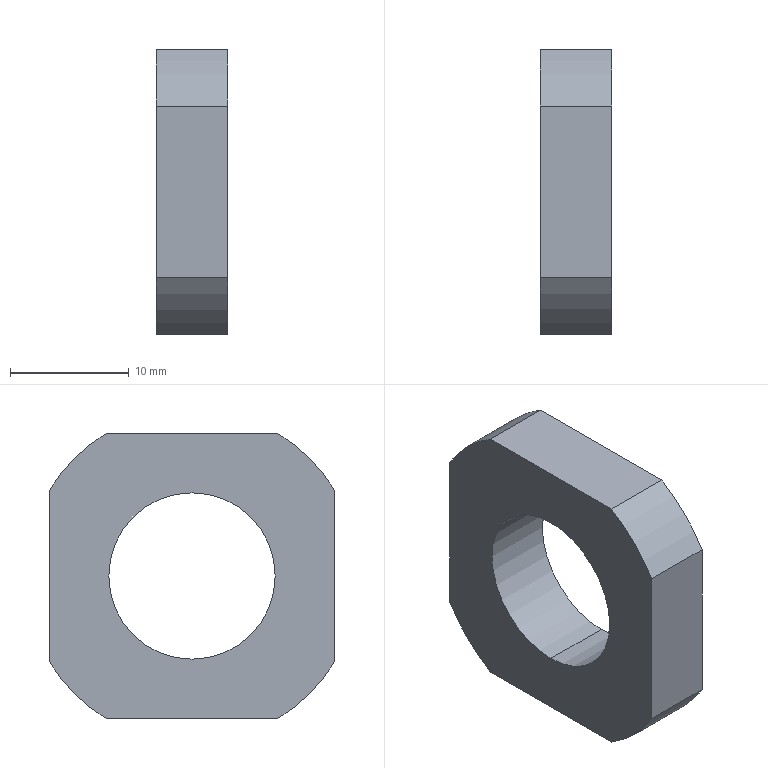Part | STEP file | PN_0053 locking nut | 1 solid | 12 faces | box 6 x 24 x 24 mm | volume 2302 mm3 | cylinder 6 | plane 6 | commonest cylinder face diameters 28 x4 14 x2
STEP:
#1=CARTESIAN_POINT('',(0.,0.,0.));
#2=DIRECTION('',(0.,0.,1.));
#3=DIRECTION('',(1.,0.,0.));
#4=AXIS2_PLACEMENT_3D('',#1,#2,#3);
#5=CARTESIAN_POINT('',(0.,0.,7.));
#6=VERTEX_POINT('',#5);
#7=CARTESIAN_POINT('',(-6.,0.,7.));
#8=VERTEX_POINT('',#7);
#9=CARTESIAN_POINT('',(0.,0.,7.));
#10=DIRECTION('',(-1.,0.,0.));
#11=VECTOR('',#10,1.);
#12=LINE('',#9,#11);
#13=CARTESIAN_POINT('',(0.,0.,0.));
#14=DIRECTION('',(-1.,0.,0.));
#15=DIRECTION('',(0.,0.,1.));
#16=AXIS2_PLACEMENT_3D('',#13,#14,#15);
#17=CYLINDRICAL_SURFACE('',#16,7.);
#18=CARTESIAN_POINT('',(6.283,0.));
#19=DIRECTION('',(0.,1.));
#20=VECTOR('',#19,1.);
#21=LINE('',#18,#20);
#22=(GEOMETRIC_REPRESENTATION_CONTEXT(2)PARAMETRIC_REPRESENTATION_CONTEXT()REPRESENTATION_CONTEXT('',''));
#23=DEFINITIONAL_REPRESENTATION('',(#21),#22);
#24=PCURVE('',#17,#23);
#25=CARTESIAN_POINT('',(0.,0.,0.));
#26=DIRECTION('',(-1.,0.,0.));
#27=DIRECTION('',(0.,0.,1.));
#28=AXIS2_PLACEMENT_3D('',#25,#26,#27);
#29=CYLINDRICAL_SURFACE('',#28,7.);
#30=CARTESIAN_POINT('',(0.,0.));
#31=DIRECTION('',(0.,1.));
#32=VECTOR('',#31,1.);
#33=LINE('',#30,#32);
#34=(GEOMETRIC_REPRESENTATION_CONTEXT(2)PARAMETRIC_REPRESENTATION_CONTEXT()REPRESENTATION_CONTEXT('',''));
#35=DEFINITIONAL_REPRESENTATION('',(#33),#34);
#36=PCURVE('',#29,#35);
#37=SURFACE_CURVE('',#12,(#24,#36),.PCURVE_S1.);
#38=EDGE_CURVE('',#6,#8,#37,.T.);
#39=ORIENTED_EDGE('',*,*,#38,.T.);
#40=CARTESIAN_POINT('',(-6.,0.,-7.));
#41=VERTEX_POINT('',#40);
#42=CARTESIAN_POINT('',(-6.,0.,0.));
#43=DIRECTION('',(1.,0.,0.));
#44=DIRECTION('',(0.,0.,-1.));
#45=AXIS2_PLACEMENT_3D('',#42,#43,#44);
#46=CIRCLE('',#45,7.);
#47=CARTESIAN_POINT('',(9.425,6.));
#48=DIRECTION('',(-1.,0.));
#49=VECTOR('',#48,1.);
#50=LINE('',#47,#49);
#51=(GEOMETRIC_REPRESENTATION_CONTEXT(2)PARAMETRIC_REPRESENTATION_CONTEXT()REPRESENTATION_CONTEXT('',''));
#52=DEFINITIONAL_REPRESENTATION('',(#50),#51);
#53=PCURVE('',#17,#52);
#54=CARTESIAN_POINT('',(-6.,14.,0.));
#55=DIRECTION('',(-1.,0.,0.));
#56=DIRECTION('',(0.,0.,1.));
#57=AXIS2_PLACEMENT_3D('',#54,#55,#56);
#58=PLANE('',#57);
#59=CARTESIAN_POINT('',(-7.,-14.));
#60=CARTESIAN_POINT('',(-7.,-1.876));
#61=CARTESIAN_POINT('',(3.5,-7.938));
#62=CARTESIAN_POINT('',(14.,-14.));
#63=CARTESIAN_POINT('',(3.5,-20.062));
#64=CARTESIAN_POINT('',(-7.,-26.124));
#65=CARTESIAN_POINT('',(-7.,-14.));
#66=(BOUNDED_CURVE()B_SPLINE_CURVE(2,(#59,#60,#61,#62,#63,#64,#65),.UNSPECIFIED.,.T.,.F.)B_SPLINE_CURVE_WITH_KNOTS((1,2,2,2,2,1),(-2.094,0.,2.094,4.189,6.283,8.378),.UNSPECIFIED.)CURVE()GEOMETRIC_REPRESENTATION_ITEM()RATIONAL_B_SPLINE_CURVE((1.,0.5,1.,0.5,1.,0.5,1.))REPRESENTATION_ITEM(''));
#67=(GEOMETRIC_REPRESENTATION_CONTEXT(2)PARAMETRIC_REPRESENTATION_CONTEXT()REPRESENTATION_CONTEXT('',''));
#68=DEFINITIONAL_REPRESENTATION('',(#66),#67);
#69=PCURVE('',#58,#68);
#70=SURFACE_CURVE('',#46,(#53,#69),.PCURVE_S1.);
#71=EDGE_CURVE('',#8,#41,#70,.T.);
#72=ORIENTED_EDGE('',*,*,#71,.T.);
#73=CARTESIAN_POINT('',(0.,0.,-7.));
#74=VERTEX_POINT('',#73);
#75=CARTESIAN_POINT('',(0.,0.,-7.));
#76=DIRECTION('',(-1.,0.,0.));
#77=VECTOR('',#76,1.);
#78=LINE('',#75,#77);
#79=CARTESIAN_POINT('',(3.142,0.));
#80=DIRECTION('',(0.,1.));
#81=VECTOR('',#80,1.);
#82=LINE('',#79,#81);
#83=(GEOMETRIC_REPRESENTATION_CONTEXT(2)PARAMETRIC_REPRESENTATION_CONTEXT()REPRESENTATION_CONTEXT('',''));
#84=DEFINITIONAL_REPRESENTATION('',(#82),#83);
#85=PCURVE('',#17,#84);
#86=CARTESIAN_POINT('',(3.142,0.));
#87=DIRECTION('',(0.,1.));
#88=VECTOR('',#87,1.);
#89=LINE('',#86,#88);
#90=(GEOMETRIC_REPRESENTATION_CONTEXT(2)PARAMETRIC_REPRESENTATION_CONTEXT()REPRESENTATION_CONTEXT('',''));
#91=DEFINITIONAL_REPRESENTATION('',(#89),#90);
#92=PCURVE('',#29,#91);
#93=SURFACE_CURVE('',#78,(#85,#92),.PCURVE_S1.);
#94=EDGE_CURVE('',#74,#41,#93,.T.);
#95=ORIENTED_EDGE('',*,*,#94,.F.);
#96=CARTESIAN_POINT('',(0.,0.,0.));
#97=DIRECTION('',(1.,0.,0.));
#98=DIRECTION('',(0.,0.,-1.));
#99=AXIS2_PLACEMENT_3D('',#96,#97,#98);
#100=CIRCLE('',#99,7.);
#101=CARTESIAN_POINT('',(9.425,0.));
#102=DIRECTION('',(-1.,0.));
#103=VECTOR('',#102,1.);
#104=LINE('',#101,#103);
#105=(GEOMETRIC_REPRESENTATION_CONTEXT(2)PARAMETRIC_REPRESENTATION_CONTEXT()REPRESENTATION_CONTEXT('',''));
#106=DEFINITIONAL_REPRESENTATION('',(#104),#105);
#107=PCURVE('',#17,#106);
#108=CARTESIAN_POINT('',(0.,0.,0.));
#109=DIRECTION('',(1.,0.,0.));
#110=DIRECTION('',(0.,0.,-1.));
#111=AXIS2_PLACEMENT_3D('',#108,#109,#110);
#112=PLANE('',#111);
#113=CARTESIAN_POINT('',(0.,0.));
#114=DIRECTION('',(1.,0.));
#115=AXIS2_PLACEMENT_2D('',#113,#114);
#116=CIRCLE('',#115,7.);
#117=(GEOMETRIC_REPRESENTATION_CONTEXT(2)PARAMETRIC_REPRESENTATION_CONTEXT()REPRESENTATION_CONTEXT('',''));
#118=DEFINITIONAL_REPRESENTATION('',(#116),#117);
#119=PCURVE('',#112,#118);
#120=SURFACE_CURVE('',#100,(#107,#119),.PCURVE_S1.);
#121=EDGE_CURVE('',#6,#74,#120,.T.);
#122=ORIENTED_EDGE('',*,*,#121,.F.);
#123=EDGE_LOOP('',(#39,#72,#95,#122));
#124=FACE_BOUND('',#123,.F.);
#125=ADVANCED_FACE('',(#124),#17,.F.);
#126=CARTESIAN_POINT('',(0.,7.211,12.));
#127=VERTEX_POINT('',#126);
#128=CARTESIAN_POINT('',(-6.,7.211,12.));
#129=VERTEX_POINT('',#128);
#130=CARTESIAN_POINT('',(0.,7.211,12.));
#131=DIRECTION('',(-1.,0.,0.));
#132=VECTOR('',#131,1.);
#133=LINE('',#130,#132);
#134=CARTESIAN_POINT('',(0.,0.,0.));
#135=DIRECTION('',(1.,0.,0.));
#136=DIRECTION('',(0.,0.,-1.));
#137=AXIS2_PLACEMENT_3D('',#134,#135,#136);
#138=CYLINDRICAL_SURFACE('',#137,14.);
#139=CARTESIAN_POINT('',(2.6,0.));
#140=DIRECTION('',(0.,-1.));
#141=VECTOR('',#140,1.);
#142=LINE('',#139,#141);
#143=(GEOMETRIC_REPRESENTATION_CONTEXT(2)PARAMETRIC_REPRESENTATION_CONTEXT()REPRESENTATION_CONTEXT('',''));
#144=DEFINITIONAL_REPRESENTATION('',(#142),#143);
#145=PCURVE('',#138,#144);
#146=CARTESIAN_POINT('',(0.,17.205,12.));
#147=DIRECTION('',(0.,0.,-1.));
#148=DIRECTION('',(0.,1.,0.));
#149=AXIS2_PLACEMENT_3D('',#146,#147,#148);
#150=PLANE('',#149);
#151=CARTESIAN_POINT('',(-9.994,0.));
#152=DIRECTION('',(0.,-1.));
#153=VECTOR('',#152,1.);
#154=LINE('',#151,#153);
#155=(GEOMETRIC_REPRESENTATION_CONTEXT(2)PARAMETRIC_REPRESENTATION_CONTEXT()REPRESENTATION_CONTEXT('',''));
#156=DEFINITIONAL_REPRESENTATION('',(#154),#155);
#157=PCURVE('',#150,#156);
#158=SURFACE_CURVE('',#133,(#145,#157),.PCURVE_S1.);
#159=EDGE_CURVE('',#127,#129,#158,.T.);
#160=ORIENTED_EDGE('',*,*,#159,.F.);
#161=CARTESIAN_POINT('',(0.,12.,7.211));
#162=VERTEX_POINT('',#161);
#163=CARTESIAN_POINT('',(0.,0.,0.));
#164=DIRECTION('',(1.,0.,0.));
#165=DIRECTION('',(0.,0.,-1.));
#166=AXIS2_PLACEMENT_3D('',#163,#164,#165);
#167=CIRCLE('',#166,14.);
#168=CARTESIAN_POINT('',(0.,0.));
#169=DIRECTION('',(1.,0.));
#170=VECTOR('',#169,1.);
#171=LINE('',#168,#170);
#172=(GEOMETRIC_REPRESENTATION_CONTEXT(2)PARAMETRIC_REPRESENTATION_CONTEXT()REPRESENTATION_CONTEXT('',''));
#173=DEFINITIONAL_REPRESENTATION('',(#171),#172);
#174=PCURVE('',#138,#173);
#175=CARTESIAN_POINT('',(0.,0.));
#176=DIRECTION('',(1.,0.));
#177=AXIS2_PLACEMENT_2D('',#175,#176);
#178=CIRCLE('',#177,14.);
#179=(GEOMETRIC_REPRESENTATION_CONTEXT(2)PARAMETRIC_REPRESENTATION_CONTEXT()REPRESENTATION_CONTEXT('',''));
#180=DEFINITIONAL_REPRESENTATION('',(#178),#179);
#181=PCURVE('',#112,#180);
#182=SURFACE_CURVE('',#167,(#174,#181),.PCURVE_S1.);
#183=EDGE_CURVE('',#162,#127,#182,.T.);
#184=ORIENTED_EDGE('',*,*,#183,.F.);
#185=CARTESIAN_POINT('',(-6.,12.,7.211));
#186=VERTEX_POINT('',#185);
#187=CARTESIAN_POINT('',(0.,12.,7.211));
#188=DIRECTION('',(1.,0.,0.));
#189=VECTOR('',#188,1.);
#190=LINE('',#187,#189);
#191=CARTESIAN_POINT('',(2.112,0.));
#192=DIRECTION('',(0.,1.));
#193=VECTOR('',#192,1.);
#194=LINE('',#191,#193);
#195=(GEOMETRIC_REPRESENTATION_CONTEXT(2)PARAMETRIC_REPRESENTATION_CONTEXT()REPRESENTATION_CONTEXT('',''));
#196=DEFINITIONAL_REPRESENTATION('',(#194),#195);
#197=PCURVE('',#138,#196);
#198=CARTESIAN_POINT('',(0.,12.,-20.296));
#199=DIRECTION('',(0.,-1.,0.));
#200=DIRECTION('',(0.,0.,-1.));
#201=AXIS2_PLACEMENT_3D('',#198,#199,#200);
#202=PLANE('',#201);
#203=CARTESIAN_POINT('',(-27.507,0.));
#204=DIRECTION('',(0.,1.));
#205=VECTOR('',#204,1.);
#206=LINE('',#203,#205);
#207=(GEOMETRIC_REPRESENTATION_CONTEXT(2)PARAMETRIC_REPRESENTATION_CONTEXT()REPRESENTATION_CONTEXT('',''));
#208=DEFINITIONAL_REPRESENTATION('',(#206),#207);
#209=PCURVE('',#202,#208);
#210=SURFACE_CURVE('',#190,(#197,#209),.PCURVE_S1.);
#211=EDGE_CURVE('',#186,#162,#210,.T.);
#212=ORIENTED_EDGE('',*,*,#211,.F.);
#213=CARTESIAN_POINT('',(-6.,0.,0.));
#214=DIRECTION('',(1.,0.,0.));
#215=DIRECTION('',(0.,0.,-1.));
#216=AXIS2_PLACEMENT_3D('',#213,#214,#215);
#217=CIRCLE('',#216,14.);
#218=CARTESIAN_POINT('',(0.,-6.));
#219=DIRECTION('',(1.,0.));
#220=VECTOR('',#219,1.);
#221=LINE('',#218,#220);
#222=(GEOMETRIC_REPRESENTATION_CONTEXT(2)PARAMETRIC_REPRESENTATION_CONTEXT()REPRESENTATION_CONTEXT('',''));
#223=DEFINITIONAL_REPRESENTATION('',(#221),#222);
#224=PCURVE('',#138,#223);
#225=CARTESIAN_POINT('',(-14.,-14.));
#226=CARTESIAN_POINT('',(-14.,10.249));
#227=CARTESIAN_POINT('',(7.,-1.876));
#228=CARTESIAN_POINT('',(28.,-14.));
#229=CARTESIAN_POINT('',(7.,-26.124));
#230=CARTESIAN_POINT('',(-14.,-38.249));
#231=CARTESIAN_POINT('',(-14.,-14.));
#232=(BOUNDED_CURVE()B_SPLINE_CURVE(2,(#225,#226,#227,#228,#229,#230,#231),.UNSPECIFIED.,.T.,.F.)B_SPLINE_CURVE_WITH_KNOTS((1,2,2,2,2,1),(-2.094,0.,2.094,4.189,6.283,8.378),.UNSPECIFIED.)CURVE()GEOMETRIC_REPRESENTATION_ITEM()RATIONAL_B_SPLINE_CURVE((1.,0.5,1.,0.5,1.,0.5,1.))REPRESENTATION_ITEM(''));
#233=(GEOMETRIC_REPRESENTATION_CONTEXT(2)PARAMETRIC_REPRESENTATION_CONTEXT()REPRESENTATION_CONTEXT('',''));
#234=DEFINITIONAL_REPRESENTATION('',(#232),#233);
#235=PCURVE('',#58,#234);
#236=SURFACE_CURVE('',#217,(#224,#235),.PCURVE_S1.);
#237=EDGE_CURVE('',#186,#129,#236,.T.);
#238=ORIENTED_EDGE('',*,*,#237,.T.);
#239=EDGE_LOOP('',(#160,#184,#212,#238));
#240=FACE_BOUND('',#239,.T.);
#241=ADVANCED_FACE('',(#240),#138,.T.);
#242=CARTESIAN_POINT('',(0.,-7.211,-12.));
#243=VERTEX_POINT('',#242);
#244=CARTESIAN_POINT('',(-6.,-7.211,-12.));
#245=VERTEX_POINT('',#244);
#246=CARTESIAN_POINT('',(0.,-7.211,-12.));
#247=DIRECTION('',(-1.,0.,0.));
#248=VECTOR('',#247,1.);
#249=LINE('',#246,#248);
#250=CARTESIAN_POINT('',(0.,0.,0.));
#251=DIRECTION('',(1.,0.,0.));
#252=DIRECTION('',(0.,0.,-1.));
#253=AXIS2_PLACEMENT_3D('',#250,#251,#252);
#254=CYLINDRICAL_SURFACE('',#253,14.);
#255=CARTESIAN_POINT('',(5.742,0.));
#256=DIRECTION('',(0.,-1.));
#257=VECTOR('',#256,1.);
#258=LINE('',#255,#257);
#259=(GEOMETRIC_REPRESENTATION_CONTEXT(2)PARAMETRIC_REPRESENTATION_CONTEXT()REPRESENTATION_CONTEXT('',''));
#260=DEFINITIONAL_REPRESENTATION('',(#258),#259);
#261=PCURVE('',#254,#260);
#262=CARTESIAN_POINT('',(0.,17.205,-12.));
#263=DIRECTION('',(0.,0.,1.));
#264=DIRECTION('',(0.,-1.,0.));
#265=AXIS2_PLACEMENT_3D('',#262,#263,#264);
#266=PLANE('',#265);
#267=CARTESIAN_POINT('',(24.416,0.));
#268=DIRECTION('',(0.,-1.));
#269=VECTOR('',#268,1.);
#270=LINE('',#267,#269);
#271=(GEOMETRIC_REPRESENTATION_CONTEXT(2)PARAMETRIC_REPRESENTATION_CONTEXT()REPRESENTATION_CONTEXT('',''));
#272=DEFINITIONAL_REPRESENTATION('',(#270),#271);
#273=PCURVE('',#266,#272);
#274=SURFACE_CURVE('',#249,(#261,#273),.PCURVE_S1.);
#275=EDGE_CURVE('',#243,#245,#274,.T.);
#276=ORIENTED_EDGE('',*,*,#275,.F.);
#277=CARTESIAN_POINT('',(0.,-12.,-7.211));
#278=VERTEX_POINT('',#277);
#279=CARTESIAN_POINT('',(0.,0.,0.));
#280=DIRECTION('',(1.,0.,0.));
#281=DIRECTION('',(0.,0.,-1.));
#282=AXIS2_PLACEMENT_3D('',#279,#280,#281);
#283=CIRCLE('',#282,14.);
#284=CARTESIAN_POINT('',(0.,0.));
#285=DIRECTION('',(1.,0.));
#286=VECTOR('',#285,1.);
#287=LINE('',#284,#286);
#288=(GEOMETRIC_REPRESENTATION_CONTEXT(2)PARAMETRIC_REPRESENTATION_CONTEXT()REPRESENTATION_CONTEXT('',''));
#289=DEFINITIONAL_REPRESENTATION('',(#287),#288);
#290=PCURVE('',#254,#289);
#291=CARTESIAN_POINT('',(0.,0.));
#292=DIRECTION('',(1.,0.));
#293=AXIS2_PLACEMENT_2D('',#291,#292);
#294=CIRCLE('',#293,14.);
#295=(GEOMETRIC_REPRESENTATION_CONTEXT(2)PARAMETRIC_REPRESENTATION_CONTEXT()REPRESENTATION_CONTEXT('',''));
#296=DEFINITIONAL_REPRESENTATION('',(#294),#295);
#297=PCURVE('',#112,#296);
#298=SURFACE_CURVE('',#283,(#290,#297),.PCURVE_S1.);
#299=EDGE_CURVE('',#278,#243,#298,.T.);
#300=ORIENTED_EDGE('',*,*,#299,.F.);
#301=CARTESIAN_POINT('',(-6.,-12.,-7.211));
#302=VERTEX_POINT('',#301);
#303=CARTESIAN_POINT('',(0.,-12.,-7.211));
#304=DIRECTION('',(1.,0.,0.));
#305=VECTOR('',#304,1.);
#306=LINE('',#303,#305);
#307=CARTESIAN_POINT('',(5.253,0.));
#308=DIRECTION('',(0.,1.));
#309=VECTOR('',#308,1.);
#310=LINE('',#307,#309);
#311=(GEOMETRIC_REPRESENTATION_CONTEXT(2)PARAMETRIC_REPRESENTATION_CONTEXT()REPRESENTATION_CONTEXT('',''));
#312=DEFINITIONAL_REPRESENTATION('',(#310),#311);
#313=PCURVE('',#254,#312);
#314=CARTESIAN_POINT('',(0.,-12.,-20.296));
#315=DIRECTION('',(0.,1.,0.));
#316=DIRECTION('',(0.,0.,1.));
#317=AXIS2_PLACEMENT_3D('',#314,#315,#316);
#318=PLANE('',#317);
#319=CARTESIAN_POINT('',(13.085,0.));
#320=DIRECTION('',(0.,1.));
#321=VECTOR('',#320,1.);
#322=LINE('',#319,#321);
#323=(GEOMETRIC_REPRESENTATION_CONTEXT(2)PARAMETRIC_REPRESENTATION_CONTEXT()REPRESENTATION_CONTEXT('',''));
#324=DEFINITIONAL_REPRESENTATION('',(#322),#323);
#325=PCURVE('',#318,#324);
#326=SURFACE_CURVE('',#306,(#313,#325),.PCURVE_S1.);
#327=EDGE_CURVE('',#302,#278,#326,.T.);
#328=ORIENTED_EDGE('',*,*,#327,.F.);
#329=CARTESIAN_POINT('',(-6.,0.,0.));
#330=DIRECTION('',(1.,0.,0.));
#331=DIRECTION('',(0.,0.,-1.));
#332=AXIS2_PLACEMENT_3D('',#329,#330,#331);
#333=CIRCLE('',#332,14.);
#334=CARTESIAN_POINT('',(0.,-6.));
#335=DIRECTION('',(1.,0.));
#336=VECTOR('',#335,1.);
#337=LINE('',#334,#336);
#338=(GEOMETRIC_REPRESENTATION_CONTEXT(2)PARAMETRIC_REPRESENTATION_CONTEXT()REPRESENTATION_CONTEXT('',''));
#339=DEFINITIONAL_REPRESENTATION('',(#337),#338);
#340=PCURVE('',#254,#339);
#341=CARTESIAN_POINT('',(-14.,-14.));
#342=CARTESIAN_POINT('',(-14.,10.249));
#343=CARTESIAN_POINT('',(7.,-1.876));
#344=CARTESIAN_POINT('',(28.,-14.));
#345=CARTESIAN_POINT('',(7.,-26.124));
#346=CARTESIAN_POINT('',(-14.,-38.249));
#347=CARTESIAN_POINT('',(-14.,-14.));
#348=(BOUNDED_CURVE()B_SPLINE_CURVE(2,(#341,#342,#343,#344,#345,#346,#347),.UNSPECIFIED.,.T.,.F.)B_SPLINE_CURVE_WITH_KNOTS((1,2,2,2,2,1),(-2.094,0.,2.094,4.189,6.283,8.378),.UNSPECIFIED.)CURVE()GEOMETRIC_REPRESENTATION_ITEM()RATIONAL_B_SPLINE_CURVE((1.,0.5,1.,0.5,1.,0.5,1.))REPRESENTATION_ITEM(''));
#349=(GEOMETRIC_REPRESENTATION_CONTEXT(2)PARAMETRIC_REPRESENTATION_CONTEXT()REPRESENTATION_CONTEXT('',''));
#350=DEFINITIONAL_REPRESENTATION('',(#348),#349);
#351=PCURVE('',#58,#350);
#352=SURFACE_CURVE('',#333,(#340,#351),.PCURVE_S1.);
#353=EDGE_CURVE('',#302,#245,#352,.T.);
#354=ORIENTED_EDGE('',*,*,#353,.T.);
#355=EDGE_LOOP('',(#276,#300,#328,#354));
#356=FACE_BOUND('',#355,.T.);
#357=ADVANCED_FACE('',(#356),#254,.T.);
#358=CARTESIAN_POINT('',(-6.,-7.211,12.));
#359=VERTEX_POINT('',#358);
#360=CARTESIAN_POINT('',(0.,-7.211,12.));
#361=VERTEX_POINT('',#360);
#362=CARTESIAN_POINT('',(0.,-7.211,12.));
#363=DIRECTION('',(1.,0.,0.));
#364=VECTOR('',#363,1.);
#365=LINE('',#362,#364);
#366=CARTESIAN_POINT('',(0.,0.,0.));
#367=DIRECTION('',(1.,0.,0.));
#368=DIRECTION('',(0.,0.,-1.));
#369=AXIS2_PLACEMENT_3D('',#366,#367,#368);
#370=CYLINDRICAL_SURFACE('',#369,14.);
#371=CARTESIAN_POINT('',(3.683,0.));
#372=DIRECTION('',(0.,1.));
#373=VECTOR('',#372,1.);
#374=LINE('',#371,#373);
#375=(GEOMETRIC_REPRESENTATION_CONTEXT(2)PARAMETRIC_REPRESENTATION_CONTEXT()REPRESENTATION_CONTEXT('',''));
#376=DEFINITIONAL_REPRESENTATION('',(#374),#375);
#377=PCURVE('',#370,#376);
#378=CARTESIAN_POINT('',(-24.416,0.));
#379=DIRECTION('',(0.,1.));
#380=VECTOR('',#379,1.);
#381=LINE('',#378,#380);
#382=(GEOMETRIC_REPRESENTATION_CONTEXT(2)PARAMETRIC_REPRESENTATION_CONTEXT()REPRESENTATION_CONTEXT('',''));
#383=DEFINITIONAL_REPRESENTATION('',(#381),#382);
#384=PCURVE('',#150,#383);
#385=SURFACE_CURVE('',#365,(#377,#384),.PCURVE_S1.);
#386=EDGE_CURVE('',#359,#361,#385,.T.);
#387=ORIENTED_EDGE('',*,*,#386,.F.);
#388=CARTESIAN_POINT('',(-6.,-12.,7.211));
#389=VERTEX_POINT('',#388);
#390=CARTESIAN_POINT('',(-6.,0.,0.));
#391=DIRECTION('',(1.,0.,0.));
#392=DIRECTION('',(0.,0.,-1.));
#393=AXIS2_PLACEMENT_3D('',#390,#391,#392);
#394=CIRCLE('',#393,14.);
#395=CARTESIAN_POINT('',(0.,-6.));
#396=DIRECTION('',(1.,0.));
#397=VECTOR('',#396,1.);
#398=LINE('',#395,#397);
#399=(GEOMETRIC_REPRESENTATION_CONTEXT(2)PARAMETRIC_REPRESENTATION_CONTEXT()REPRESENTATION_CONTEXT('',''));
#400=DEFINITIONAL_REPRESENTATION('',(#398),#399);
#401=PCURVE('',#370,#400);
#402=CARTESIAN_POINT('',(-14.,-14.));
#403=CARTESIAN_POINT('',(-14.,10.249));
#404=CARTESIAN_POINT('',(7.,-1.876));
#405=CARTESIAN_POINT('',(28.,-14.));
#406=CARTESIAN_POINT('',(7.,-26.124));
#407=CARTESIAN_POINT('',(-14.,-38.249));
#408=CARTESIAN_POINT('',(-14.,-14.));
#409=(BOUNDED_CURVE()B_SPLINE_CURVE(2,(#402,#403,#404,#405,#406,#407,#408),.UNSPECIFIED.,.T.,.F.)B_SPLINE_CURVE_WITH_KNOTS((1,2,2,2,2,1),(-2.094,0.,2.094,4.189,6.283,8.378),.UNSPECIFIED.)CURVE()GEOMETRIC_REPRESENTATION_ITEM()RATIONAL_B_SPLINE_CURVE((1.,0.5,1.,0.5,1.,0.5,1.))REPRESENTATION_ITEM(''));
#410=(GEOMETRIC_REPRESENTATION_CONTEXT(2)PARAMETRIC_REPRESENTATION_CONTEXT()REPRESENTATION_CONTEXT('',''));
#411=DEFINITIONAL_REPRESENTATION('',(#409),#410);
#412=PCURVE('',#58,#411);
#413=SURFACE_CURVE('',#394,(#401,#412),.PCURVE_S1.);
#414=EDGE_CURVE('',#359,#389,#413,.T.);
#415=ORIENTED_EDGE('',*,*,#414,.T.);
#416=CARTESIAN_POINT('',(0.,-12.,7.211));
#417=VERTEX_POINT('',#416);
#418=CARTESIAN_POINT('',(0.,-12.,7.211));
#419=DIRECTION('',(-1.,0.,0.));
#420=VECTOR('',#419,1.);
#421=LINE('',#418,#420);
#422=CARTESIAN_POINT('',(4.171,0.));
#423=DIRECTION('',(0.,-1.));
#424=VECTOR('',#423,1.);
#425=LINE('',#422,#424);
#426=(GEOMETRIC_REPRESENTATION_CONTEXT(2)PARAMETRIC_REPRESENTATION_CONTEXT()REPRESENTATION_CONTEXT('',''));
#427=DEFINITIONAL_REPRESENTATION('',(#425),#426);
#428=PCURVE('',#370,#427);
#429=CARTESIAN_POINT('',(27.507,0.));
#430=DIRECTION('',(0.,-1.));
#431=VECTOR('',#430,1.);
#432=LINE('',#429,#431);
#433=(GEOMETRIC_REPRESENTATION_CONTEXT(2)PARAMETRIC_REPRESENTATION_CONTEXT()REPRESENTATION_CONTEXT('',''));
#434=DEFINITIONAL_REPRESENTATION('',(#432),#433);
#435=PCURVE('',#318,#434);
#436=SURFACE_CURVE('',#421,(#428,#435),.PCURVE_S1.);
#437=EDGE_CURVE('',#417,#389,#436,.T.);
#438=ORIENTED_EDGE('',*,*,#437,.F.);
#439=CARTESIAN_POINT('',(0.,0.,0.));
#440=DIRECTION('',(1.,0.,0.));
#441=DIRECTION('',(0.,0.,-1.));
#442=AXIS2_PLACEMENT_3D('',#439,#440,#441);
#443=CIRCLE('',#442,14.);
#444=CARTESIAN_POINT('',(0.,0.));
#445=DIRECTION('',(1.,0.));
#446=VECTOR('',#445,1.);
#447=LINE('',#444,#446);
#448=(GEOMETRIC_REPRESENTATION_CONTEXT(2)PARAMETRIC_REPRESENTATION_CONTEXT()REPRESENTATION_CONTEXT('',''));
#449=DEFINITIONAL_REPRESENTATION('',(#447),#448);
#450=PCURVE('',#370,#449);
#451=CARTESIAN_POINT('',(0.,0.));
#452=DIRECTION('',(1.,0.));
#453=AXIS2_PLACEMENT_2D('',#451,#452);
#454=CIRCLE('',#453,14.);
#455=(GEOMETRIC_REPRESENTATION_CONTEXT(2)PARAMETRIC_REPRESENTATION_CONTEXT()REPRESENTATION_CONTEXT('',''));
#456=DEFINITIONAL_REPRESENTATION('',(#454),#455);
#457=PCURVE('',#112,#456);
#458=SURFACE_CURVE('',#443,(#450,#457),.PCURVE_S1.);
#459=EDGE_CURVE('',#361,#417,#458,.T.);
#460=ORIENTED_EDGE('',*,*,#459,.F.);
#461=EDGE_LOOP('',(#387,#415,#438,#460));
#462=FACE_BOUND('',#461,.T.);
#463=ADVANCED_FACE('',(#462),#370,.T.);
#464=CARTESIAN_POINT('',(0.,17.205,12.));
#465=DIRECTION('',(0.,-1.,0.));
#466=VECTOR('',#465,1.);
#467=LINE('',#464,#466);
#468=CARTESIAN_POINT('',(-12.,17.205));
#469=DIRECTION('',(0.,-1.));
#470=VECTOR('',#469,1.);
#471=LINE('',#468,#470);
#472=(GEOMETRIC_REPRESENTATION_CONTEXT(2)PARAMETRIC_REPRESENTATION_CONTEXT()REPRESENTATION_CONTEXT('',''));
#473=DEFINITIONAL_REPRESENTATION('',(#471),#472);
#474=PCURVE('',#112,#473);
#475=CARTESIAN_POINT('',(0.,0.));
#476=DIRECTION('',(-1.,0.));
#477=VECTOR('',#476,1.);
#478=LINE('',#475,#477);
#479=(GEOMETRIC_REPRESENTATION_CONTEXT(2)PARAMETRIC_REPRESENTATION_CONTEXT()REPRESENTATION_CONTEXT('',''));
#480=DEFINITIONAL_REPRESENTATION('',(#478),#479);
#481=PCURVE('',#150,#480);
#482=SURFACE_CURVE('',#467,(#474,#481),.PCURVE_S1.);
#483=EDGE_CURVE('',#127,#361,#482,.T.);
#484=ORIENTED_EDGE('',*,*,#483,.T.);
#485=ORIENTED_EDGE('',*,*,#459,.T.);
#486=CARTESIAN_POINT('',(0.,-12.,-20.296));
#487=DIRECTION('',(0.,0.,-1.));
#488=VECTOR('',#487,1.);
#489=LINE('',#486,#488);
#490=CARTESIAN_POINT('',(20.296,-12.));
#491=DIRECTION('',(1.,0.));
#492=VECTOR('',#491,1.);
#493=LINE('',#490,#492);
#494=(GEOMETRIC_REPRESENTATION_CONTEXT(2)PARAMETRIC_REPRESENTATION_CONTEXT()REPRESENTATION_CONTEXT('',''));
#495=DEFINITIONAL_REPRESENTATION('',(#493),#494);
#496=PCURVE('',#112,#495);
#497=CARTESIAN_POINT('',(0.,0.));
#498=DIRECTION('',(-1.,0.));
#499=VECTOR('',#498,1.);
#500=LINE('',#497,#499);
#501=(GEOMETRIC_REPRESENTATION_CONTEXT(2)PARAMETRIC_REPRESENTATION_CONTEXT()REPRESENTATION_CONTEXT('',''));
#502=DEFINITIONAL_REPRESENTATION('',(#500),#501);
#503=PCURVE('',#318,#502);
#504=SURFACE_CURVE('',#489,(#496,#503),.PCURVE_S1.);
#505=EDGE_CURVE('',#417,#278,#504,.T.);
#506=ORIENTED_EDGE('',*,*,#505,.T.);
#507=ORIENTED_EDGE('',*,*,#299,.T.);
#508=CARTESIAN_POINT('',(0.,7.211,-12.));
#509=VERTEX_POINT('',#508);
#510=CARTESIAN_POINT('',(0.,17.205,-12.));
#511=DIRECTION('',(0.,1.,0.));
#512=VECTOR('',#511,1.);
#513=LINE('',#510,#512);
#514=CARTESIAN_POINT('',(12.,17.205));
#515=DIRECTION('',(0.,1.));
#516=VECTOR('',#515,1.);
#517=LINE('',#514,#516);
#518=(GEOMETRIC_REPRESENTATION_CONTEXT(2)PARAMETRIC_REPRESENTATION_CONTEXT()REPRESENTATION_CONTEXT('',''));
#519=DEFINITIONAL_REPRESENTATION('',(#517),#518);
#520=PCURVE('',#112,#519);
#521=CARTESIAN_POINT('',(0.,0.));
#522=DIRECTION('',(-1.,0.));
#523=VECTOR('',#522,1.);
#524=LINE('',#521,#523);
#525=(GEOMETRIC_REPRESENTATION_CONTEXT(2)PARAMETRIC_REPRESENTATION_CONTEXT()REPRESENTATION_CONTEXT('',''));
#526=DEFINITIONAL_REPRESENTATION('',(#524),#525);
#527=PCURVE('',#266,#526);
#528=SURFACE_CURVE('',#513,(#520,#527),.PCURVE_S1.);
#529=EDGE_CURVE('',#243,#509,#528,.T.);
#530=ORIENTED_EDGE('',*,*,#529,.T.);
#531=CARTESIAN_POINT('',(0.,12.,-7.211));
#532=VERTEX_POINT('',#531);
#533=CARTESIAN_POINT('',(0.,0.,0.));
#534=DIRECTION('',(1.,0.,0.));
#535=DIRECTION('',(0.,0.,-1.));
#536=AXIS2_PLACEMENT_3D('',#533,#534,#535);
#537=CIRCLE('',#536,14.);
#538=CARTESIAN_POINT('',(0.,0.));
#539=DIRECTION('',(1.,0.));
#540=AXIS2_PLACEMENT_2D('',#538,#539);
#541=CIRCLE('',#540,14.);
#542=(GEOMETRIC_REPRESENTATION_CONTEXT(2)PARAMETRIC_REPRESENTATION_CONTEXT()REPRESENTATION_CONTEXT('',''));
#543=DEFINITIONAL_REPRESENTATION('',(#541),#542);
#544=PCURVE('',#112,#543);
#545=CARTESIAN_POINT('',(0.,0.,0.));
#546=DIRECTION('',(1.,0.,0.));
#547=DIRECTION('',(0.,0.,-1.));
#548=AXIS2_PLACEMENT_3D('',#545,#546,#547);
#549=CYLINDRICAL_SURFACE('',#548,14.);
#550=CARTESIAN_POINT('',(0.,0.));
#551=DIRECTION('',(1.,0.));
#552=VECTOR('',#551,1.);
#553=LINE('',#550,#552);
#554=(GEOMETRIC_REPRESENTATION_CONTEXT(2)PARAMETRIC_REPRESENTATION_CONTEXT()REPRESENTATION_CONTEXT('',''));
#555=DEFINITIONAL_REPRESENTATION('',(#553),#554);
#556=PCURVE('',#549,#555);
#557=SURFACE_CURVE('',#537,(#544,#556),.PCURVE_S1.);
#558=EDGE_CURVE('',#509,#532,#557,.T.);
#559=ORIENTED_EDGE('',*,*,#558,.T.);
#560=CARTESIAN_POINT('',(0.,12.,-20.296));
#561=DIRECTION('',(0.,0.,1.));
#562=VECTOR('',#561,1.);
#563=LINE('',#560,#562);
#564=CARTESIAN_POINT('',(20.296,12.));
#565=DIRECTION('',(-1.,0.));
#566=VECTOR('',#565,1.);
#567=LINE('',#564,#566);
#568=(GEOMETRIC_REPRESENTATION_CONTEXT(2)PARAMETRIC_REPRESENTATION_CONTEXT()REPRESENTATION_CONTEXT('',''));
#569=DEFINITIONAL_REPRESENTATION('',(#567),#568);
#570=PCURVE('',#112,#569);
#571=CARTESIAN_POINT('',(0.,0.));
#572=DIRECTION('',(-1.,0.));
#573=VECTOR('',#572,1.);
#574=LINE('',#571,#573);
#575=(GEOMETRIC_REPRESENTATION_CONTEXT(2)PARAMETRIC_REPRESENTATION_CONTEXT()REPRESENTATION_CONTEXT('',''));
#576=DEFINITIONAL_REPRESENTATION('',(#574),#575);
#577=PCURVE('',#202,#576);
#578=SURFACE_CURVE('',#563,(#570,#577),.PCURVE_S1.);
#579=EDGE_CURVE('',#532,#162,#578,.T.);
#580=ORIENTED_EDGE('',*,*,#579,.T.);
#581=ORIENTED_EDGE('',*,*,#183,.T.);
#582=EDGE_LOOP('',(#484,#485,#506,#507,#530,#559,#580,#581));
#583=FACE_BOUND('',#582,.T.);
#584=ORIENTED_EDGE('',*,*,#121,.F.);
#585=CARTESIAN_POINT('',(0.,0.,0.));
#586=DIRECTION('',(1.,0.,0.));
#587=DIRECTION('',(0.,0.,-1.));
#588=AXIS2_PLACEMENT_3D('',#585,#586,#587);
#589=CIRCLE('',#588,7.);
#590=CARTESIAN_POINT('',(0.,0.));
#591=DIRECTION('',(1.,0.));
#592=AXIS2_PLACEMENT_2D('',#590,#591);
#593=CIRCLE('',#592,7.);
#594=(GEOMETRIC_REPRESENTATION_CONTEXT(2)PARAMETRIC_REPRESENTATION_CONTEXT()REPRESENTATION_CONTEXT('',''));
#595=DEFINITIONAL_REPRESENTATION('',(#593),#594);
#596=PCURVE('',#112,#595);
#597=CARTESIAN_POINT('',(3.142,0.));
#598=DIRECTION('',(-1.,0.));
#599=VECTOR('',#598,1.);
#600=LINE('',#597,#599);
#601=(GEOMETRIC_REPRESENTATION_CONTEXT(2)PARAMETRIC_REPRESENTATION_CONTEXT()REPRESENTATION_CONTEXT('',''));
#602=DEFINITIONAL_REPRESENTATION('',(#600),#601);
#603=PCURVE('',#29,#602);
#604=SURFACE_CURVE('',#589,(#596,#603),.PCURVE_S1.);
#605=EDGE_CURVE('',#74,#6,#604,.T.);
#606=ORIENTED_EDGE('',*,*,#605,.F.);
#607=EDGE_LOOP('',(#584,#606));
#608=FACE_BOUND('',#607,.T.);
#609=ADVANCED_FACE('',(#583,#608),#112,.T.);
#610=CARTESIAN_POINT('',(-6.,14.,12.));
#611=DIRECTION('',(0.,-1.,0.));
#612=VECTOR('',#611,1.);
#613=LINE('',#610,#612);
#614=CARTESIAN_POINT('',(12.,0.));
#615=DIRECTION('',(0.,-1.));
#616=VECTOR('',#615,1.);
#617=LINE('',#614,#616);
#618=(GEOMETRIC_REPRESENTATION_CONTEXT(2)PARAMETRIC_REPRESENTATION_CONTEXT()REPRESENTATION_CONTEXT('',''));
#619=DEFINITIONAL_REPRESENTATION('',(#617),#618);
#620=PCURVE('',#58,#619);
#621=CARTESIAN_POINT('',(-3.205,-6.));
#622=DIRECTION('',(-1.,0.));
#623=VECTOR('',#622,1.);
#624=LINE('',#621,#623);
#625=(GEOMETRIC_REPRESENTATION_CONTEXT(2)PARAMETRIC_REPRESENTATION_CONTEXT()REPRESENTATION_CONTEXT('',''));
#626=DEFINITIONAL_REPRESENTATION('',(#624),#625);
#627=PCURVE('',#150,#626);
#628=SURFACE_CURVE('',#613,(#620,#627),.PCURVE_S1.);
#629=EDGE_CURVE('',#129,#359,#628,.T.);
#630=ORIENTED_EDGE('',*,*,#629,.F.);
#631=ORIENTED_EDGE('',*,*,#237,.F.);
#632=CARTESIAN_POINT('',(-6.,12.,-7.211));
#633=VERTEX_POINT('',#632);
#634=CARTESIAN_POINT('',(-6.,12.,-20.296));
#635=DIRECTION('',(0.,0.,1.));
#636=VECTOR('',#635,1.);
#637=LINE('',#634,#636);
#638=CARTESIAN_POINT('',(-20.296,-2.));
#639=DIRECTION('',(1.,0.));
#640=VECTOR('',#639,1.);
#641=LINE('',#638,#640);
#642=(GEOMETRIC_REPRESENTATION_CONTEXT(2)PARAMETRIC_REPRESENTATION_CONTEXT()REPRESENTATION_CONTEXT('',''));
#643=DEFINITIONAL_REPRESENTATION('',(#641),#642);
#644=PCURVE('',#58,#643);
#645=CARTESIAN_POINT('',(0.,-6.));
#646=DIRECTION('',(-1.,0.));
#647=VECTOR('',#646,1.);
#648=LINE('',#645,#647);
#649=(GEOMETRIC_REPRESENTATION_CONTEXT(2)PARAMETRIC_REPRESENTATION_CONTEXT()REPRESENTATION_CONTEXT('',''));
#650=DEFINITIONAL_REPRESENTATION('',(#648),#649);
#651=PCURVE('',#202,#650);
#652=SURFACE_CURVE('',#637,(#644,#651),.PCURVE_S1.);
#653=EDGE_CURVE('',#633,#186,#652,.T.);
#654=ORIENTED_EDGE('',*,*,#653,.F.);
#655=CARTESIAN_POINT('',(-6.,7.211,-12.));
#656=VERTEX_POINT('',#655);
#657=CARTESIAN_POINT('',(-6.,0.,0.));
#658=DIRECTION('',(1.,0.,0.));
#659=DIRECTION('',(0.,0.,-1.));
#660=AXIS2_PLACEMENT_3D('',#657,#658,#659);
#661=CIRCLE('',#660,14.);
#662=CARTESIAN_POINT('',(-14.,-14.));
#663=CARTESIAN_POINT('',(-14.,10.249));
#664=CARTESIAN_POINT('',(7.,-1.876));
#665=CARTESIAN_POINT('',(28.,-14.));
#666=CARTESIAN_POINT('',(7.,-26.124));
#667=CARTESIAN_POINT('',(-14.,-38.249));
#668=CARTESIAN_POINT('',(-14.,-14.));
#669=(BOUNDED_CURVE()B_SPLINE_CURVE(2,(#662,#663,#664,#665,#666,#667,#668),.UNSPECIFIED.,.T.,.F.)B_SPLINE_CURVE_WITH_KNOTS((1,2,2,2,2,1),(-2.094,0.,2.094,4.189,6.283,8.378),.UNSPECIFIED.)CURVE()GEOMETRIC_REPRESENTATION_ITEM()RATIONAL_B_SPLINE_CURVE((1.,0.5,1.,0.5,1.,0.5,1.))REPRESENTATION_ITEM(''));
#670=(GEOMETRIC_REPRESENTATION_CONTEXT(2)PARAMETRIC_REPRESENTATION_CONTEXT()REPRESENTATION_CONTEXT('',''));
#671=DEFINITIONAL_REPRESENTATION('',(#669),#670);
#672=PCURVE('',#58,#671);
#673=CARTESIAN_POINT('',(0.,-6.));
#674=DIRECTION('',(1.,0.));
#675=VECTOR('',#674,1.);
#676=LINE('',#673,#675);
#677=(GEOMETRIC_REPRESENTATION_CONTEXT(2)PARAMETRIC_REPRESENTATION_CONTEXT()REPRESENTATION_CONTEXT('',''));
#678=DEFINITIONAL_REPRESENTATION('',(#676),#677);
#679=PCURVE('',#549,#678);
#680=SURFACE_CURVE('',#661,(#672,#679),.PCURVE_S1.);
#681=EDGE_CURVE('',#656,#633,#680,.T.);
#682=ORIENTED_EDGE('',*,*,#681,.F.);
#683=CARTESIAN_POINT('',(-6.,17.205,-12.));
#684=DIRECTION('',(0.,1.,0.));
#685=VECTOR('',#684,1.);
#686=LINE('',#683,#685);
#687=CARTESIAN_POINT('',(-12.,3.205));
#688=DIRECTION('',(0.,1.));
#689=VECTOR('',#688,1.);
#690=LINE('',#687,#689);
#691=(GEOMETRIC_REPRESENTATION_CONTEXT(2)PARAMETRIC_REPRESENTATION_CONTEXT()REPRESENTATION_CONTEXT('',''));
#692=DEFINITIONAL_REPRESENTATION('',(#690),#691);
#693=PCURVE('',#58,#692);
#694=CARTESIAN_POINT('',(0.,-6.));
#695=DIRECTION('',(-1.,0.));
#696=VECTOR('',#695,1.);
#697=LINE('',#694,#696);
#698=(GEOMETRIC_REPRESENTATION_CONTEXT(2)PARAMETRIC_REPRESENTATION_CONTEXT()REPRESENTATION_CONTEXT('',''));
#699=DEFINITIONAL_REPRESENTATION('',(#697),#698);
#700=PCURVE('',#266,#699);
#701=SURFACE_CURVE('',#686,(#693,#700),.PCURVE_S1.);
#702=EDGE_CURVE('',#245,#656,#701,.T.);
#703=ORIENTED_EDGE('',*,*,#702,.F.);
#704=ORIENTED_EDGE('',*,*,#353,.F.);
#705=CARTESIAN_POINT('',(-6.,-12.,-20.296));
#706=DIRECTION('',(0.,0.,-1.));
#707=VECTOR('',#706,1.);
#708=LINE('',#705,#707);
#709=CARTESIAN_POINT('',(-20.296,-26.));
#710=DIRECTION('',(-1.,0.));
#711=VECTOR('',#710,1.);
#712=LINE('',#709,#711);
#713=(GEOMETRIC_REPRESENTATION_CONTEXT(2)PARAMETRIC_REPRESENTATION_CONTEXT()REPRESENTATION_CONTEXT('',''));
#714=DEFINITIONAL_REPRESENTATION('',(#712),#713);
#715=PCURVE('',#58,#714);
#716=CARTESIAN_POINT('',(0.,-6.));
#717=DIRECTION('',(-1.,0.));
#718=VECTOR('',#717,1.);
#719=LINE('',#716,#718);
#720=(GEOMETRIC_REPRESENTATION_CONTEXT(2)PARAMETRIC_REPRESENTATION_CONTEXT()REPRESENTATION_CONTEXT('',''));
#721=DEFINITIONAL_REPRESENTATION('',(#719),#720);
#722=PCURVE('',#318,#721);
#723=SURFACE_CURVE('',#708,(#715,#722),.PCURVE_S1.);
#724=EDGE_CURVE('',#389,#302,#723,.T.);
#725=ORIENTED_EDGE('',*,*,#724,.F.);
#726=ORIENTED_EDGE('',*,*,#414,.F.);
#727=EDGE_LOOP('',(#630,#631,#654,#682,#703,#704,#725,#726));
#728=FACE_BOUND('',#727,.T.);
#729=ORIENTED_EDGE('',*,*,#71,.T.);
#730=CARTESIAN_POINT('',(-6.,0.,0.));
#731=DIRECTION('',(1.,0.,0.));
#732=DIRECTION('',(0.,0.,-1.));
#733=AXIS2_PLACEMENT_3D('',#730,#731,#732);
#734=CIRCLE('',#733,7.);
#735=CARTESIAN_POINT('',(-7.,-14.));
#736=CARTESIAN_POINT('',(-7.,-1.876));
#737=CARTESIAN_POINT('',(3.5,-7.938));
#738=CARTESIAN_POINT('',(14.,-14.));
#739=CARTESIAN_POINT('',(3.5,-20.062));
#740=CARTESIAN_POINT('',(-7.,-26.124));
#741=CARTESIAN_POINT('',(-7.,-14.));
#742=(BOUNDED_CURVE()B_SPLINE_CURVE(2,(#735,#736,#737,#738,#739,#740,#741),.UNSPECIFIED.,.T.,.F.)B_SPLINE_CURVE_WITH_KNOTS((1,2,2,2,2,1),(-2.094,0.,2.094,4.189,6.283,8.378),.UNSPECIFIED.)CURVE()GEOMETRIC_REPRESENTATION_ITEM()RATIONAL_B_SPLINE_CURVE((1.,0.5,1.,0.5,1.,0.5,1.))REPRESENTATION_ITEM(''));
#743=(GEOMETRIC_REPRESENTATION_CONTEXT(2)PARAMETRIC_REPRESENTATION_CONTEXT()REPRESENTATION_CONTEXT('',''));
#744=DEFINITIONAL_REPRESENTATION('',(#742),#743);
#745=PCURVE('',#58,#744);
#746=CARTESIAN_POINT('',(3.142,6.));
#747=DIRECTION('',(-1.,0.));
#748=VECTOR('',#747,1.);
#749=LINE('',#746,#748);
#750=(GEOMETRIC_REPRESENTATION_CONTEXT(2)PARAMETRIC_REPRESENTATION_CONTEXT()REPRESENTATION_CONTEXT('',''));
#751=DEFINITIONAL_REPRESENTATION('',(#749),#750);
#752=PCURVE('',#29,#751);
#753=SURFACE_CURVE('',#734,(#745,#752),.PCURVE_S1.);
#754=EDGE_CURVE('',#41,#8,#753,.T.);
#755=ORIENTED_EDGE('',*,*,#754,.T.);
#756=EDGE_LOOP('',(#729,#755));
#757=FACE_BOUND('',#756,.T.);
#758=ADVANCED_FACE('',(#728,#757),#58,.T.);
#759=CARTESIAN_POINT('',(0.,7.211,-12.));
#760=DIRECTION('',(1.,0.,0.));
#761=VECTOR('',#760,1.);
#762=LINE('',#759,#761);
#763=CARTESIAN_POINT('',(0.5411,0.));
#764=DIRECTION('',(0.,1.));
#765=VECTOR('',#764,1.);
#766=LINE('',#763,#765);
#767=(GEOMETRIC_REPRESENTATION_CONTEXT(2)PARAMETRIC_REPRESENTATION_CONTEXT()REPRESENTATION_CONTEXT('',''));
#768=DEFINITIONAL_REPRESENTATION('',(#766),#767);
#769=PCURVE('',#549,#768);
#770=CARTESIAN_POINT('',(9.994,0.));
#771=DIRECTION('',(0.,1.));
#772=VECTOR('',#771,1.);
#773=LINE('',#770,#772);
#774=(GEOMETRIC_REPRESENTATION_CONTEXT(2)PARAMETRIC_REPRESENTATION_CONTEXT()REPRESENTATION_CONTEXT('',''));
#775=DEFINITIONAL_REPRESENTATION('',(#773),#774);
#776=PCURVE('',#266,#775);
#777=SURFACE_CURVE('',#762,(#769,#776),.PCURVE_S1.);
#778=EDGE_CURVE('',#656,#509,#777,.T.);
#779=ORIENTED_EDGE('',*,*,#778,.F.);
#780=ORIENTED_EDGE('',*,*,#681,.T.);
#781=CARTESIAN_POINT('',(0.,12.,-7.211));
#782=DIRECTION('',(-1.,0.,0.));
#783=VECTOR('',#782,1.);
#784=LINE('',#781,#783);
#785=CARTESIAN_POINT('',(1.03,0.));
#786=DIRECTION('',(0.,-1.));
#787=VECTOR('',#786,1.);
#788=LINE('',#785,#787);
#789=(GEOMETRIC_REPRESENTATION_CONTEXT(2)PARAMETRIC_REPRESENTATION_CONTEXT()REPRESENTATION_CONTEXT('',''));
#790=DEFINITIONAL_REPRESENTATION('',(#788),#789);
#791=PCURVE('',#549,#790);
#792=CARTESIAN_POINT('',(-13.085,0.));
#793=DIRECTION('',(0.,-1.));
#794=VECTOR('',#793,1.);
#795=LINE('',#792,#794);
#796=(GEOMETRIC_REPRESENTATION_CONTEXT(2)PARAMETRIC_REPRESENTATION_CONTEXT()REPRESENTATION_CONTEXT('',''));
#797=DEFINITIONAL_REPRESENTATION('',(#795),#796);
#798=PCURVE('',#202,#797);
#799=SURFACE_CURVE('',#784,(#791,#798),.PCURVE_S1.);
#800=EDGE_CURVE('',#532,#633,#799,.T.);
#801=ORIENTED_EDGE('',*,*,#800,.F.);
#802=ORIENTED_EDGE('',*,*,#558,.F.);
#803=EDGE_LOOP('',(#779,#780,#801,#802));
#804=FACE_BOUND('',#803,.T.);
#805=ADVANCED_FACE('',(#804),#549,.T.);
#806=ORIENTED_EDGE('',*,*,#754,.T.);
#807=ORIENTED_EDGE('',*,*,#38,.F.);
#808=ORIENTED_EDGE('',*,*,#605,.F.);
#809=ORIENTED_EDGE('',*,*,#94,.T.);
#810=EDGE_LOOP('',(#806,#807,#808,#809));
#811=FACE_BOUND('',#810,.F.);
#812=ADVANCED_FACE('',(#811),#29,.F.);
#813=ORIENTED_EDGE('',*,*,#800,.T.);
#814=ORIENTED_EDGE('',*,*,#653,.T.);
#815=ORIENTED_EDGE('',*,*,#211,.T.);
#816=ORIENTED_EDGE('',*,*,#579,.F.);
#817=EDGE_LOOP('',(#813,#814,#815,#816));
#818=FACE_BOUND('',#817,.T.);
#819=ADVANCED_FACE('',(#818),#202,.F.);
#820=ORIENTED_EDGE('',*,*,#437,.T.);
#821=ORIENTED_EDGE('',*,*,#724,.T.);
#822=ORIENTED_EDGE('',*,*,#327,.T.);
#823=ORIENTED_EDGE('',*,*,#505,.F.);
#824=EDGE_LOOP('',(#820,#821,#822,#823));
#825=FACE_BOUND('',#824,.T.);
#826=ADVANCED_FACE('',(#825),#318,.F.);
#827=ORIENTED_EDGE('',*,*,#275,.T.);
#828=ORIENTED_EDGE('',*,*,#702,.T.);
#829=ORIENTED_EDGE('',*,*,#778,.T.);
#830=ORIENTED_EDGE('',*,*,#529,.F.);
#831=EDGE_LOOP('',(#827,#828,#829,#830));
#832=FACE_BOUND('',#831,.T.);
#833=ADVANCED_FACE('',(#832),#266,.F.);
#834=ORIENTED_EDGE('',*,*,#159,.T.);
#835=ORIENTED_EDGE('',*,*,#629,.T.);
#836=ORIENTED_EDGE('',*,*,#386,.T.);
#837=ORIENTED_EDGE('',*,*,#483,.F.);
#838=EDGE_LOOP('',(#834,#835,#836,#837));
#839=FACE_BOUND('',#838,.T.);
#840=ADVANCED_FACE('',(#839),#150,.F.);
#841=CLOSED_SHELL('',(#125,#241,#357,#463,#609,#758,#805,#812,#819,#826,#833,#840));
#842=MANIFOLD_SOLID_BREP('',#841);
#843=(LENGTH_UNIT()NAMED_UNIT(*)SI_UNIT(.MILLI.,.METRE.));
#844=UNCERTAINTY_MEASURE_WITH_UNIT(LENGTH_MEASURE(0.0000001),#843,'','');
#845=(NAMED_UNIT(*)PLANE_ANGLE_UNIT()SI_UNIT($,.RADIAN.));
#846=(NAMED_UNIT(*)SI_UNIT($,.STERADIAN.)SOLID_ANGLE_UNIT());
#847=(GEOMETRIC_REPRESENTATION_CONTEXT(3)GLOBAL_UNCERTAINTY_ASSIGNED_CONTEXT((#844))GLOBAL_UNIT_ASSIGNED_CONTEXT((#843,#845,#846))REPRESENTATION_CONTEXT('',''));
#848=ADVANCED_BREP_SHAPE_REPRESENTATION('',(#4,#842),#847);